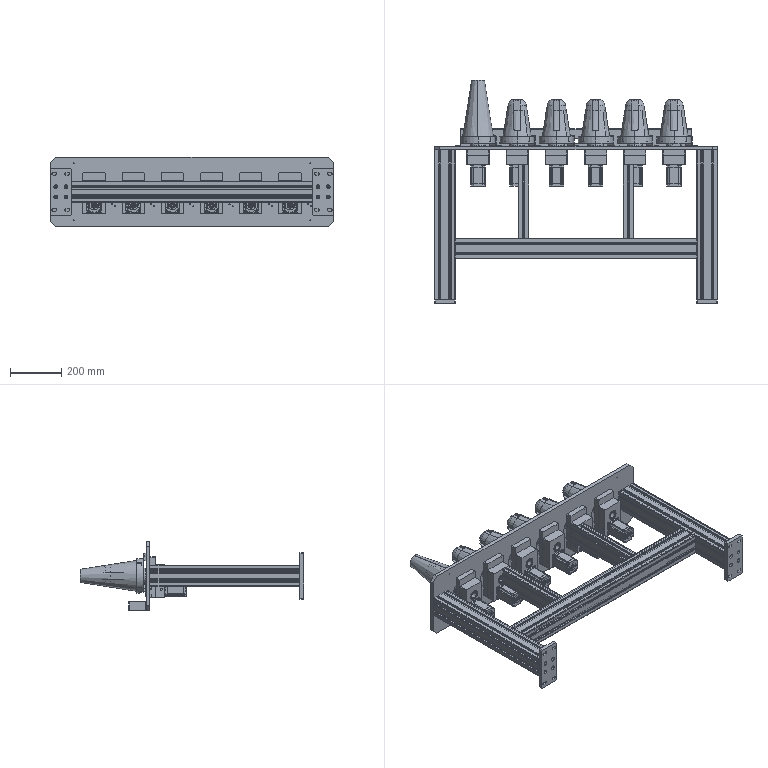Part | SolidWorks | 161 solids | 19690 faces | volume 19249167 mm3 | plane 9144 | cylinder 7142 | spline 1882 | cone 1510 | torus 12 | commonest cylinder face diameters 0.5 x1536 72 x444 67.5 x426 0.6 x372 3 x272 32.5 x210